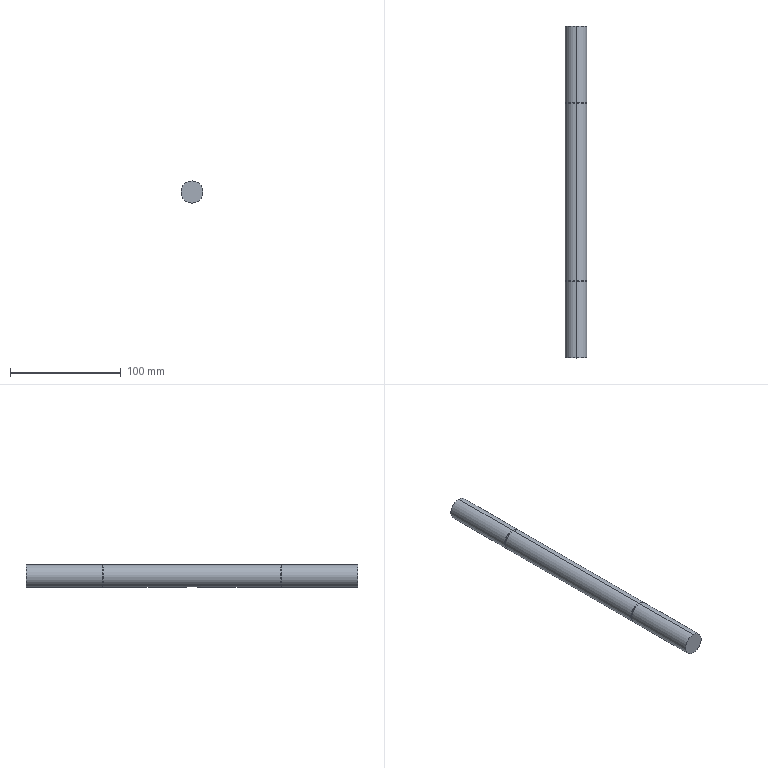Part | SolidWorks | features ICE 3, Chamfer 1, Extrusion 1 | 1 solid | 21 faces | box 20 x 300 x 20 mm | volume 93992 mm3 | cylinder 12 | plane 9 | commonest cylinder face diameters 20 x6 19 x4 6 x2
STEP:
#1=CARTESIAN_POINT('',(0.,300.,10.));
#2=VERTEX_POINT('',#1);
#3=CARTESIAN_POINT('',(0.,300.,-10.));
#4=VERTEX_POINT('',#3);
#5=CARTESIAN_POINT('',(0.,300.,0.));
#6=DIRECTION('',(0.,1.,0.));
#7=DIRECTION('',(0.,0.,1.));
#8=AXIS2_PLACEMENT_3D('',#5,#6,#7);
#9=CIRCLE('',#8,10.);
#10=EDGE_CURVE('',#2,#4,#9,.T.);
#11=ORIENTED_EDGE('',*,*,#10,.F.);
#12=CARTESIAN_POINT('',(0.,231.3,10.));
#13=VERTEX_POINT('',#12);
#14=CARTESIAN_POINT('',(0.,300.,10.));
#15=DIRECTION('',(0.,-1.,0.));
#16=VECTOR('',#15,1000.);
#17=LINE('',#14,#16);
#18=EDGE_CURVE('',#2,#13,#17,.T.);
#19=ORIENTED_EDGE('',*,*,#18,.T.);
#20=CARTESIAN_POINT('',(0.,231.3,-10.));
#21=VERTEX_POINT('',#20);
#22=CARTESIAN_POINT('',(0.,231.3,0.));
#23=DIRECTION('',(0.,1.,0.));
#24=DIRECTION('',(0.,0.,1.));
#25=AXIS2_PLACEMENT_3D('',#22,#23,#24);
#26=CIRCLE('',#25,10.);
#27=EDGE_CURVE('',#13,#21,#26,.T.);
#28=ORIENTED_EDGE('',*,*,#27,.T.);
#29=CARTESIAN_POINT('',(0.,300.,-10.));
#30=DIRECTION('',(0.,-1.,0.));
#31=VECTOR('',#30,1000.);
#32=LINE('',#29,#31);
#33=EDGE_CURVE('',#4,#21,#32,.T.);
#34=ORIENTED_EDGE('',*,*,#33,.F.);
#35=EDGE_LOOP('',(#11,#19,#28,#34));
#36=FACE_OUTER_BOUND('',#35,.T.);
#37=CARTESIAN_POINT('',(0.,300.,0.));
#38=DIRECTION('',(0.,-1.,0.));
#39=DIRECTION('',(0.,0.,-1.));
#40=AXIS2_PLACEMENT_3D('',#37,#38,#39);
#41=CYLINDRICAL_SURFACE('',#40,10.);
#42=ADVANCED_FACE('',(#36),#41,.T.);
#43=CARTESIAN_POINT('',(0.,231.3,9.5));
#44=VERTEX_POINT('',#43);
#45=CARTESIAN_POINT('',(0.,231.3,-9.5));
#46=VERTEX_POINT('',#45);
#47=CARTESIAN_POINT('',(0.,231.3,0.));
#48=DIRECTION('',(0.,1.,0.));
#49=DIRECTION('',(0.,0.,1.));
#50=AXIS2_PLACEMENT_3D('',#47,#48,#49);
#51=CIRCLE('',#50,9.5);
#52=EDGE_CURVE('',#44,#46,#51,.T.);
#53=ORIENTED_EDGE('',*,*,#52,.F.);
#54=CARTESIAN_POINT('',(0.,230.,9.5));
#55=VERTEX_POINT('',#54);
#56=CARTESIAN_POINT('',(0.,231.3,9.5));
#57=DIRECTION('',(0.,-1.,0.));
#58=VECTOR('',#57,1000.);
#59=LINE('',#56,#58);
#60=EDGE_CURVE('',#44,#55,#59,.T.);
#61=ORIENTED_EDGE('',*,*,#60,.T.);
#62=CARTESIAN_POINT('',(0.,230.,-9.5));
#63=VERTEX_POINT('',#62);
#64=CARTESIAN_POINT('',(0.,230.,0.));
#65=DIRECTION('',(0.,1.,0.));
#66=DIRECTION('',(0.,0.,1.));
#67=AXIS2_PLACEMENT_3D('',#64,#65,#66);
#68=CIRCLE('',#67,9.5);
#69=EDGE_CURVE('',#55,#63,#68,.T.);
#70=ORIENTED_EDGE('',*,*,#69,.T.);
#71=CARTESIAN_POINT('',(0.,231.3,-9.5));
#72=DIRECTION('',(0.,-1.,0.));
#73=VECTOR('',#72,1000.);
#74=LINE('',#71,#73);
#75=EDGE_CURVE('',#46,#63,#74,.T.);
#76=ORIENTED_EDGE('',*,*,#75,.F.);
#77=EDGE_LOOP('',(#53,#61,#70,#76));
#78=FACE_OUTER_BOUND('',#77,.T.);
#79=CARTESIAN_POINT('',(0.,231.3,0.));
#80=DIRECTION('',(0.,-1.,0.));
#81=DIRECTION('',(0.,0.,-1.));
#82=AXIS2_PLACEMENT_3D('',#79,#80,#81);
#83=CYLINDRICAL_SURFACE('',#82,9.5);
#84=ADVANCED_FACE('',(#78),#83,.T.);
#85=CARTESIAN_POINT('',(0.,68.7,-9.5));
#86=VERTEX_POINT('',#85);
#87=CARTESIAN_POINT('',(0.,68.7,9.5));
#88=VERTEX_POINT('',#87);
#89=CARTESIAN_POINT('',(0.,68.7,0.));
#90=DIRECTION('',(0.,-1.,0.));
#91=DIRECTION('',(0.,0.,-1.));
#92=AXIS2_PLACEMENT_3D('',#89,#90,#91);
#93=CIRCLE('',#92,9.5);
#94=EDGE_CURVE('',#86,#88,#93,.T.);
#95=ORIENTED_EDGE('',*,*,#94,.F.);
#96=CARTESIAN_POINT('',(0.,70.,-9.5));
#97=VERTEX_POINT('',#96);
#98=CARTESIAN_POINT('',(0.,68.7,-9.5));
#99=DIRECTION('',(0.,1.,0.));
#100=VECTOR('',#99,1000.);
#101=LINE('',#98,#100);
#102=EDGE_CURVE('',#86,#97,#101,.T.);
#103=ORIENTED_EDGE('',*,*,#102,.T.);
#104=CARTESIAN_POINT('',(0.,70.,9.5));
#105=VERTEX_POINT('',#104);
#106=CARTESIAN_POINT('',(0.,70.,0.));
#107=DIRECTION('',(0.,-1.,0.));
#108=DIRECTION('',(0.,0.,-1.));
#109=AXIS2_PLACEMENT_3D('',#106,#107,#108);
#110=CIRCLE('',#109,9.5);
#111=EDGE_CURVE('',#97,#105,#110,.T.);
#112=ORIENTED_EDGE('',*,*,#111,.T.);
#113=CARTESIAN_POINT('',(0.,68.7,9.5));
#114=DIRECTION('',(0.,1.,0.));
#115=VECTOR('',#114,1000.);
#116=LINE('',#113,#115);
#117=EDGE_CURVE('',#88,#105,#116,.T.);
#118=ORIENTED_EDGE('',*,*,#117,.F.);
#119=EDGE_LOOP('',(#95,#103,#112,#118));
#120=FACE_OUTER_BOUND('',#119,.T.);
#121=CARTESIAN_POINT('',(0.,68.7,0.));
#122=DIRECTION('',(0.,1.,0.));
#123=DIRECTION('',(0.,0.,1.));
#124=AXIS2_PLACEMENT_3D('',#121,#122,#123);
#125=CYLINDRICAL_SURFACE('',#124,9.5);
#126=ADVANCED_FACE('',(#120),#125,.T.);
#127=CARTESIAN_POINT('',(0.,68.7,-10.));
#128=VERTEX_POINT('',#127);
#129=CARTESIAN_POINT('',(0.,68.7,10.));
#130=VERTEX_POINT('',#129);
#131=CARTESIAN_POINT('',(0.,68.7,0.));
#132=DIRECTION('',(0.,-1.,0.));
#133=DIRECTION('',(0.,0.,-1.));
#134=AXIS2_PLACEMENT_3D('',#131,#132,#133);
#135=CIRCLE('',#134,10.);
#136=EDGE_CURVE('',#128,#130,#135,.T.);
#137=ORIENTED_EDGE('',*,*,#136,.T.);
#138=CARTESIAN_POINT('',(0.,0.,10.));
#139=VERTEX_POINT('',#138);
#140=CARTESIAN_POINT('',(0.,300.,10.));
#141=DIRECTION('',(0.,-1.,0.));
#142=VECTOR('',#141,1000.);
#143=LINE('',#140,#142);
#144=EDGE_CURVE('',#130,#139,#143,.T.);
#145=ORIENTED_EDGE('',*,*,#144,.T.);
#146=CARTESIAN_POINT('',(0.,0.,-10.));
#147=VERTEX_POINT('',#146);
#148=CARTESIAN_POINT('',(0.,0.,0.));
#149=DIRECTION('',(0.,1.,0.));
#150=DIRECTION('',(0.,0.,1.));
#151=AXIS2_PLACEMENT_3D('',#148,#149,#150);
#152=CIRCLE('',#151,10.);
#153=EDGE_CURVE('',#139,#147,#152,.T.);
#154=ORIENTED_EDGE('',*,*,#153,.T.);
#155=CARTESIAN_POINT('',(0.,300.,-10.));
#156=DIRECTION('',(0.,-1.,0.));
#157=VECTOR('',#156,1000.);
#158=LINE('',#155,#157);
#159=EDGE_CURVE('',#128,#147,#158,.T.);
#160=ORIENTED_EDGE('',*,*,#159,.F.);
#161=EDGE_LOOP('',(#137,#145,#154,#160));
#162=FACE_OUTER_BOUND('',#161,.T.);
#163=CARTESIAN_POINT('',(0.,300.,0.));
#164=DIRECTION('',(0.,-1.,0.));
#165=DIRECTION('',(0.,0.,-1.));
#166=AXIS2_PLACEMENT_3D('',#163,#164,#165);
#167=CYLINDRICAL_SURFACE('',#166,10.);
#168=ADVANCED_FACE('',(#162),#167,.T.);
#169=CARTESIAN_POINT('',(0.,230.,10.));
#170=VERTEX_POINT('',#169);
#171=CARTESIAN_POINT('',(0.,230.,-10.));
#172=VERTEX_POINT('',#171);
#173=CARTESIAN_POINT('',(0.,230.,0.));
#174=DIRECTION('',(0.,1.,0.));
#175=DIRECTION('',(0.,0.,1.));
#176=AXIS2_PLACEMENT_3D('',#173,#174,#175);
#177=CIRCLE('',#176,10.);
#178=EDGE_CURVE('',#170,#172,#177,.T.);
#179=ORIENTED_EDGE('',*,*,#178,.F.);
#180=CARTESIAN_POINT('',(0.,70.,10.));
#181=VERTEX_POINT('',#180);
#182=CARTESIAN_POINT('',(0.,300.,10.));
#183=DIRECTION('',(0.,-1.,0.));
#184=VECTOR('',#183,1000.);
#185=LINE('',#182,#184);
#186=EDGE_CURVE('',#170,#181,#185,.T.);
#187=ORIENTED_EDGE('',*,*,#186,.T.);
#188=CARTESIAN_POINT('',(0.,70.,-10.));
#189=VERTEX_POINT('',#188);
#190=CARTESIAN_POINT('',(0.,70.,0.));
#191=DIRECTION('',(0.,-1.,0.));
#192=DIRECTION('',(0.,0.,-1.));
#193=AXIS2_PLACEMENT_3D('',#190,#191,#192);
#194=CIRCLE('',#193,10.);
#195=EDGE_CURVE('',#189,#181,#194,.T.);
#196=ORIENTED_EDGE('',*,*,#195,.F.);
#197=CARTESIAN_POINT('',(0.,145.,-10.));
#198=VERTEX_POINT('',#197);
#199=CARTESIAN_POINT('',(0.,300.,-10.));
#200=DIRECTION('',(0.,-1.,0.));
#201=VECTOR('',#200,1000.);
#202=LINE('',#199,#201);
#203=EDGE_CURVE('',#198,#189,#202,.T.);
#204=ORIENTED_EDGE('',*,*,#203,.F.);
#205=CARTESIAN_POINT('',(3.,148.,-9.539));
#206=VERTEX_POINT('',#205);
#207=CARTESIAN_POINT('',(0.,145.,-10.));
#208=CARTESIAN_POINT('',(0.1968,145.,-10.));
#209=CARTESIAN_POINT('',(0.3967,145.02,-9.994));
#210=CARTESIAN_POINT('',(0.7821,145.097,-9.971));
#211=CARTESIAN_POINT('',(0.9695,145.154,-9.955));
#212=CARTESIAN_POINT('',(1.334,145.306,-9.912));
#213=CARTESIAN_POINT('',(1.507,145.399,-9.887));
#214=CARTESIAN_POINT('',(1.831,145.616,-9.832));
#215=CARTESIAN_POINT('',(1.983,145.741,-9.802));
#216=CARTESIAN_POINT('',(2.26,146.017,-9.742));
#217=CARTESIAN_POINT('',(2.383,146.167,-9.713));
#218=CARTESIAN_POINT('',(2.6,146.491,-9.657));
#219=CARTESIAN_POINT('',(2.694,146.667,-9.63));
#220=CARTESIAN_POINT('',(2.845,147.028,-9.587));
#221=CARTESIAN_POINT('',(2.902,147.215,-9.57));
#222=CARTESIAN_POINT('',(2.98,147.601,-9.546));
#223=CARTESIAN_POINT('',(3.,147.801,-9.539));
#224=CARTESIAN_POINT('',(3.,148.,-9.539));
#225=B_SPLINE_CURVE_WITH_KNOTS('',3,(#207,#208,#209,#210,#211,#212,#213,#214,#215,#216,#217,#218,#219,#220,#221,#222,#223,#224),.UNSPECIFIED.,.F.,.F.,(4,2,2,2,2,2,2,2,4),(0.004718,0.005307,0.005896,0.006485,0.007074,0.007663,0.008252,0.008842,0.009431),.UNSPECIFIED.);
#226=EDGE_CURVE('',#198,#206,#225,.T.);
#227=ORIENTED_EDGE('',*,*,#226,.T.);
#228=CARTESIAN_POINT('',(3.,152.,-9.539));
#229=VERTEX_POINT('',#228);
#230=CARTESIAN_POINT('',(3.,300.,-9.539));
#231=DIRECTION('',(0.,1.,0.));
#232=VECTOR('',#231,1000.);
#233=LINE('',#230,#232);
#234=EDGE_CURVE('',#206,#229,#233,.T.);
#235=ORIENTED_EDGE('',*,*,#234,.T.);
#236=CARTESIAN_POINT('',(0.,155.,-10.));
#237=VERTEX_POINT('',#236);
#238=CARTESIAN_POINT('',(3.,152.,-9.539));
#239=CARTESIAN_POINT('',(3.,152.2,-9.539));
#240=CARTESIAN_POINT('',(2.98,152.395,-9.546));
#241=CARTESIAN_POINT('',(2.903,152.781,-9.569));
#242=CARTESIAN_POINT('',(2.845,152.972,-9.587));
#243=CARTESIAN_POINT('',(2.694,153.335,-9.631));
#244=CARTESIAN_POINT('',(2.602,153.506,-9.656));
#245=CARTESIAN_POINT('',(2.384,153.832,-9.712));
#246=CARTESIAN_POINT('',(2.258,153.985,-9.743));
#247=CARTESIAN_POINT('',(1.845,154.397,-9.832));
#248=CARTESIAN_POINT('',(1.512,154.62,-9.892));
#249=CARTESIAN_POINT('',(0.971,154.845,-9.954));
#250=CARTESIAN_POINT('',(0.7806,154.903,-9.971));
#251=CARTESIAN_POINT('',(0.3926,154.981,-9.994));
#252=CARTESIAN_POINT('',(0.197,155.,-10.));
#253=CARTESIAN_POINT('',(0.,155.,-10.));
#254=B_SPLINE_CURVE_WITH_KNOTS('',3,(#238,#239,#240,#241,#242,#243,#244,#245,#246,#247,#248,#249,#250,#251,#252,#253),.UNSPECIFIED.,.F.,.F.,(4,2,2,2,2,2,2,4),(0.,0.0005898,0.00118,0.001769,0.002359,0.003539,0.004128,0.004718),.UNSPECIFIED.);
#255=EDGE_CURVE('',#229,#237,#254,.T.);
#256=ORIENTED_EDGE('',*,*,#255,.T.);
#257=CARTESIAN_POINT('',(0.,300.,-10.));
#258=DIRECTION('',(0.,-1.,0.));
#259=VECTOR('',#258,1000.);
#260=LINE('',#257,#259);
#261=EDGE_CURVE('',#172,#237,#260,.T.);
#262=ORIENTED_EDGE('',*,*,#261,.F.);
#263=EDGE_LOOP('',(#179,#187,#196,#204,#227,#235,#256,#262));
#264=FACE_OUTER_BOUND('',#263,.T.);
#265=CARTESIAN_POINT('',(0.,300.,0.));
#266=DIRECTION('',(0.,-1.,0.));
#267=DIRECTION('',(0.,0.,-1.));
#268=AXIS2_PLACEMENT_3D('',#265,#266,#267);
#269=CYLINDRICAL_SURFACE('',#268,10.);
#270=ADVANCED_FACE('',(#264),#269,.T.);
#271=ORIENTED_EDGE('',*,*,#186,.F.);
#272=CARTESIAN_POINT('',(0.,230.,0.));
#273=DIRECTION('',(0.,1.,0.));
#274=DIRECTION('',(0.,0.,1.));
#275=AXIS2_PLACEMENT_3D('',#272,#273,#274);
#276=CIRCLE('',#275,10.);
#277=EDGE_CURVE('',#172,#170,#276,.T.);
#278=ORIENTED_EDGE('',*,*,#277,.F.);
#279=ORIENTED_EDGE('',*,*,#261,.T.);
#280=CARTESIAN_POINT('',(-3.,152.,-9.539));
#281=VERTEX_POINT('',#280);
#282=CARTESIAN_POINT('',(0.,155.,-10.));
#283=CARTESIAN_POINT('',(-0.1968,155.,-10.));
#284=CARTESIAN_POINT('',(-0.3967,154.98,-9.994));
#285=CARTESIAN_POINT('',(-0.7821,154.903,-9.971));
#286=CARTESIAN_POINT('',(-0.9695,154.846,-9.955));
#287=CARTESIAN_POINT('',(-1.334,154.694,-9.912));
#288=CARTESIAN_POINT('',(-1.507,154.601,-9.887));
#289=CARTESIAN_POINT('',(-1.831,154.384,-9.832));
#290=CARTESIAN_POINT('',(-1.983,154.259,-9.802));
#291=CARTESIAN_POINT('',(-2.26,153.983,-9.742));
#292=CARTESIAN_POINT('',(-2.383,153.833,-9.713));
#293=CARTESIAN_POINT('',(-2.6,153.509,-9.657));
#294=CARTESIAN_POINT('',(-2.694,153.333,-9.63));
#295=CARTESIAN_POINT('',(-2.845,152.972,-9.587));
#296=CARTESIAN_POINT('',(-2.902,152.785,-9.57));
#297=CARTESIAN_POINT('',(-2.98,152.399,-9.546));
#298=CARTESIAN_POINT('',(-3.,152.199,-9.539));
#299=CARTESIAN_POINT('',(-3.,152.,-9.539));
#300=B_SPLINE_CURVE_WITH_KNOTS('',3,(#282,#283,#284,#285,#286,#287,#288,#289,#290,#291,#292,#293,#294,#295,#296,#297,#298,#299),.UNSPECIFIED.,.F.,.F.,(4,2,2,2,2,2,2,2,4),(0.004718,0.005307,0.005896,0.006485,0.007074,0.007663,0.008252,0.008842,0.009431),.UNSPECIFIED.);
#301=EDGE_CURVE('',#237,#281,#300,.T.);
#302=ORIENTED_EDGE('',*,*,#301,.T.);
#303=CARTESIAN_POINT('',(-3.,148.,-9.539));
#304=VERTEX_POINT('',#303);
#305=CARTESIAN_POINT('',(-3.,300.,-9.539));
#306=DIRECTION('',(0.,-1.,0.));
#307=VECTOR('',#306,1000.);
#308=LINE('',#305,#307);
#309=EDGE_CURVE('',#281,#304,#308,.T.);
#310=ORIENTED_EDGE('',*,*,#309,.T.);
#311=CARTESIAN_POINT('',(-3.,148.,-9.539));
#312=CARTESIAN_POINT('',(-3.,147.8,-9.539));
#313=CARTESIAN_POINT('',(-2.98,147.605,-9.546));
#314=CARTESIAN_POINT('',(-2.903,147.219,-9.569));
#315=CARTESIAN_POINT('',(-2.845,147.028,-9.587));
#316=CARTESIAN_POINT('',(-2.694,146.665,-9.631));
#317=CARTESIAN_POINT('',(-2.602,146.494,-9.656));
#318=CARTESIAN_POINT('',(-2.384,146.168,-9.712));
#319=CARTESIAN_POINT('',(-2.258,146.015,-9.743));
#320=CARTESIAN_POINT('',(-1.845,145.603,-9.832));
#321=CARTESIAN_POINT('',(-1.512,145.38,-9.892));
#322=CARTESIAN_POINT('',(-0.971,145.155,-9.954));
#323=CARTESIAN_POINT('',(-0.7806,145.097,-9.971));
#324=CARTESIAN_POINT('',(-0.3926,145.019,-9.994));
#325=CARTESIAN_POINT('',(-0.197,145.,-10.));
#326=CARTESIAN_POINT('',(0.,145.,-10.));
#327=B_SPLINE_CURVE_WITH_KNOTS('',3,(#311,#312,#313,#314,#315,#316,#317,#318,#319,#320,#321,#322,#323,#324,#325,#326),.UNSPECIFIED.,.F.,.F.,(4,2,2,2,2,2,2,4),(0.,0.0005898,0.00118,0.001769,0.002359,0.003539,0.004128,0.004718),.UNSPECIFIED.);
#328=EDGE_CURVE('',#304,#198,#327,.T.);
#329=ORIENTED_EDGE('',*,*,#328,.T.);
#330=ORIENTED_EDGE('',*,*,#203,.T.);
#331=CARTESIAN_POINT('',(0.,70.,0.));
#332=DIRECTION('',(0.,-1.,0.));
#333=DIRECTION('',(0.,0.,-1.));
#334=AXIS2_PLACEMENT_3D('',#331,#332,#333);
#335=CIRCLE('',#334,10.);
#336=EDGE_CURVE('',#181,#189,#335,.T.);
#337=ORIENTED_EDGE('',*,*,#336,.F.);
#338=EDGE_LOOP('',(#271,#278,#279,#302,#310,#329,#330,#337));
#339=FACE_OUTER_BOUND('',#338,.T.);
#340=CARTESIAN_POINT('',(0.,300.,0.));
#341=DIRECTION('',(0.,-1.,0.));
#342=DIRECTION('',(0.,0.,-1.));
#343=AXIS2_PLACEMENT_3D('',#340,#341,#342);
#344=CYLINDRICAL_SURFACE('',#343,10.);
#345=ADVANCED_FACE('',(#339),#344,.T.);
#346=ORIENTED_EDGE('',*,*,#144,.F.);
#347=CARTESIAN_POINT('',(0.,68.7,0.));
#348=DIRECTION('',(0.,-1.,0.));
#349=DIRECTION('',(0.,0.,-1.));
#350=AXIS2_PLACEMENT_3D('',#347,#348,#349);
#351=CIRCLE('',#350,10.);
#352=EDGE_CURVE('',#130,#128,#351,.T.);
#353=ORIENTED_EDGE('',*,*,#352,.T.);
#354=ORIENTED_EDGE('',*,*,#159,.T.);
#355=CARTESIAN_POINT('',(0.,0.,0.));
#356=DIRECTION('',(0.,1.,0.));
#357=DIRECTION('',(0.,0.,1.));
#358=AXIS2_PLACEMENT_3D('',#355,#356,#357);
#359=CIRCLE('',#358,10.);
#360=EDGE_CURVE('',#147,#139,#359,.T.);
#361=ORIENTED_EDGE('',*,*,#360,.T.);
#362=EDGE_LOOP('',(#346,#353,#354,#361));
#363=FACE_OUTER_BOUND('',#362,.T.);
#364=CARTESIAN_POINT('',(0.,300.,0.));
#365=DIRECTION('',(0.,-1.,0.));
#366=DIRECTION('',(0.,0.,-1.));
#367=AXIS2_PLACEMENT_3D('',#364,#365,#366);
#368=CYLINDRICAL_SURFACE('',#367,10.);
#369=ADVANCED_FACE('',(#363),#368,.T.);
#370=ORIENTED_EDGE('',*,*,#360,.F.);
#371=ORIENTED_EDGE('',*,*,#153,.F.);
#372=EDGE_LOOP('',(#370,#371));
#373=FACE_OUTER_BOUND('',#372,.T.);
#374=CARTESIAN_POINT('',(0.,0.,0.));
#375=DIRECTION('',(0.,1.,0.));
#376=DIRECTION('',(0.,0.,1.));
#377=AXIS2_PLACEMENT_3D('',#374,#375,#376);
#378=PLANE('',#377);
#379=ADVANCED_FACE('',(#373),#378,.F.);
#380=ORIENTED_EDGE('',*,*,#136,.F.);
#381=ORIENTED_EDGE('',*,*,#352,.F.);
#382=EDGE_LOOP('',(#380,#381));
#383=FACE_OUTER_BOUND('',#382,.T.);
#384=CARTESIAN_POINT('',(0.,68.7,0.));
#385=DIRECTION('',(0.,-1.,0.));
#386=DIRECTION('',(0.,0.,-1.));
#387=AXIS2_PLACEMENT_3D('',#384,#385,#386);
#388=CIRCLE('',#387,9.5);
#389=EDGE_CURVE('',#88,#86,#388,.T.);
#390=ORIENTED_EDGE('',*,*,#389,.T.);
#391=ORIENTED_EDGE('',*,*,#94,.T.);
#392=EDGE_LOOP('',(#390,#391));
#393=FACE_BOUND('',#392,.T.);
#394=CARTESIAN_POINT('',(0.,68.7,0.));
#395=DIRECTION('',(0.,-1.,0.));
#396=DIRECTION('',(0.,0.,-1.));
#397=AXIS2_PLACEMENT_3D('',#394,#395,#396);
#398=PLANE('',#397);
#399=ADVANCED_FACE('',(#383,#393),#398,.F.);
#400=ORIENTED_EDGE('',*,*,#195,.T.);
#401=ORIENTED_EDGE('',*,*,#336,.T.);
#402=EDGE_LOOP('',(#400,#401));
#403=FACE_OUTER_BOUND('',#402,.T.);
#404=CARTESIAN_POINT('',(0.,70.,0.));
#405=DIRECTION('',(0.,-1.,0.));
#406=DIRECTION('',(0.,0.,-1.));
#407=AXIS2_PLACEMENT_3D('',#404,#405,#406);
#408=CIRCLE('',#407,9.5);
#409=EDGE_CURVE('',#105,#97,#408,.T.);
#410=ORIENTED_EDGE('',*,*,#409,.F.);
#411=ORIENTED_EDGE('',*,*,#111,.F.);
#412=EDGE_LOOP('',(#410,#411));
#413=FACE_BOUND('',#412,.T.);
#414=CARTESIAN_POINT('',(0.,70.,0.));
#415=DIRECTION('',(0.,-1.,0.));
#416=DIRECTION('',(0.,0.,-1.));
#417=AXIS2_PLACEMENT_3D('',#414,#415,#416);
#418=PLANE('',#417);
#419=ADVANCED_FACE('',(#403,#413),#418,.T.);
#420=ORIENTED_EDGE('',*,*,#102,.F.);
#421=ORIENTED_EDGE('',*,*,#389,.F.);
#422=ORIENTED_EDGE('',*,*,#117,.T.);
#423=ORIENTED_EDGE('',*,*,#409,.T.);
#424=EDGE_LOOP('',(#420,#421,#422,#423));
#425=FACE_OUTER_BOUND('',#424,.T.);
#426=CARTESIAN_POINT('',(0.,68.7,0.));
#427=DIRECTION('',(0.,1.,0.));
#428=DIRECTION('',(0.,0.,1.));
#429=AXIS2_PLACEMENT_3D('',#426,#427,#428);
#430=CYLINDRICAL_SURFACE('',#429,9.5);
#431=ADVANCED_FACE('',(#425),#430,.T.);
#432=CARTESIAN_POINT('',(0.,231.3,0.));
#433=DIRECTION('',(0.,1.,0.));
#434=DIRECTION('',(0.,0.,1.));
#435=AXIS2_PLACEMENT_3D('',#432,#433,#434);
#436=CIRCLE('',#435,10.);
#437=EDGE_CURVE('',#21,#13,#436,.T.);
#438=ORIENTED_EDGE('',*,*,#437,.F.);
#439=ORIENTED_EDGE('',*,*,#27,.F.);
#440=EDGE_LOOP('',(#438,#439));
#441=FACE_OUTER_BOUND('',#440,.T.);
#442=CARTESIAN_POINT('',(0.,231.3,0.));
#443=DIRECTION('',(0.,1.,0.));
#444=DIRECTION('',(0.,0.,1.));
#445=AXIS2_PLACEMENT_3D('',#442,#443,#444);
#446=CIRCLE('',#445,9.5);
#447=EDGE_CURVE('',#46,#44,#446,.T.);
#448=ORIENTED_EDGE('',*,*,#447,.T.);
#449=ORIENTED_EDGE('',*,*,#52,.T.);
#450=EDGE_LOOP('',(#448,#449));
#451=FACE_BOUND('',#450,.T.);
#452=CARTESIAN_POINT('',(0.,231.3,0.));
#453=DIRECTION('',(0.,1.,0.));
#454=DIRECTION('',(0.,0.,1.));
#455=AXIS2_PLACEMENT_3D('',#452,#453,#454);
#456=PLANE('',#455);
#457=ADVANCED_FACE('',(#441,#451),#456,.F.);
#458=ORIENTED_EDGE('',*,*,#277,.T.);
#459=ORIENTED_EDGE('',*,*,#178,.T.);
#460=EDGE_LOOP('',(#458,#459));
#461=FACE_OUTER_BOUND('',#460,.T.);
#462=CARTESIAN_POINT('',(0.,230.,0.));
#463=DIRECTION('',(0.,1.,0.));
#464=DIRECTION('',(0.,0.,1.));
#465=AXIS2_PLACEMENT_3D('',#462,#463,#464);
#466=CIRCLE('',#465,9.5);
#467=EDGE_CURVE('',#63,#55,#466,.T.);
#468=ORIENTED_EDGE('',*,*,#467,.F.);
#469=ORIENTED_EDGE('',*,*,#69,.F.);
#470=EDGE_LOOP('',(#468,#469));
#471=FACE_BOUND('',#470,.T.);
#472=CARTESIAN_POINT('',(0.,230.,0.));
#473=DIRECTION('',(0.,1.,0.));
#474=DIRECTION('',(0.,0.,1.));
#475=AXIS2_PLACEMENT_3D('',#472,#473,#474);
#476=PLANE('',#475);
#477=ADVANCED_FACE('',(#461,#471),#476,.T.);
#478=ORIENTED_EDGE('',*,*,#60,.F.);
#479=ORIENTED_EDGE('',*,*,#447,.F.);
#480=ORIENTED_EDGE('',*,*,#75,.T.);
#481=ORIENTED_EDGE('',*,*,#467,.T.);
#482=EDGE_LOOP('',(#478,#479,#480,#481));
#483=FACE_OUTER_BOUND('',#482,.T.);
#484=CARTESIAN_POINT('',(0.,231.3,0.));
#485=DIRECTION('',(0.,-1.,0.));
#486=DIRECTION('',(0.,0.,-1.));
#487=AXIS2_PLACEMENT_3D('',#484,#485,#486);
#488=CYLINDRICAL_SURFACE('',#487,9.5);
#489=ADVANCED_FACE('',(#483),#488,.T.);
#490=CARTESIAN_POINT('',(0.,300.,0.));
#491=DIRECTION('',(0.,1.,0.));
#492=DIRECTION('',(0.,0.,1.));
#493=AXIS2_PLACEMENT_3D('',#490,#491,#492);
#494=CIRCLE('',#493,10.);
#495=EDGE_CURVE('',#4,#2,#494,.T.);
#496=ORIENTED_EDGE('',*,*,#495,.T.);
#497=ORIENTED_EDGE('',*,*,#10,.T.);
#498=EDGE_LOOP('',(#496,#497));
#499=FACE_OUTER_BOUND('',#498,.T.);
#500=CARTESIAN_POINT('',(0.,300.,0.));
#501=DIRECTION('',(0.,1.,0.));
#502=DIRECTION('',(0.,0.,1.));
#503=AXIS2_PLACEMENT_3D('',#500,#501,#502);
#504=PLANE('',#503);
#505=ADVANCED_FACE('',(#499),#504,.T.);
#506=ORIENTED_EDGE('',*,*,#18,.F.);
#507=ORIENTED_EDGE('',*,*,#495,.F.);
#508=ORIENTED_EDGE('',*,*,#33,.T.);
#509=ORIENTED_EDGE('',*,*,#437,.T.);
#510=EDGE_LOOP('',(#506,#507,#508,#509));
#511=FACE_OUTER_BOUND('',#510,.T.);
#512=CARTESIAN_POINT('',(0.,300.,0.));
#513=DIRECTION('',(0.,-1.,0.));
#514=DIRECTION('',(0.,0.,-1.));
#515=AXIS2_PLACEMENT_3D('',#512,#513,#514);
#516=CYLINDRICAL_SURFACE('',#515,10.);
#517=ADVANCED_FACE('',(#511),#516,.T.);
#518=CARTESIAN_POINT('',(-3.,148.,-6.5));
#519=VERTEX_POINT('',#518);
#520=CARTESIAN_POINT('',(-3.,148.,-6.5));
#521=DIRECTION('',(0.,0.,-1.));
#522=VECTOR('',#521,1000.);
#523=LINE('',#520,#522);
#524=EDGE_CURVE('',#519,#304,#523,.T.);
#525=ORIENTED_EDGE('',*,*,#524,.F.);
#526=CARTESIAN_POINT('',(3.,148.,-6.5));
#527=VERTEX_POINT('',#526);
#528=CARTESIAN_POINT('',(0.,148.,-6.5));
#529=DIRECTION('',(0.,0.,-1.));
#530=DIRECTION('',(-1.,0.,0.));
#531=AXIS2_PLACEMENT_3D('',#528,#529,#530);
#532=CIRCLE('',#531,3.);
#533=EDGE_CURVE('',#527,#519,#532,.T.);
#534=ORIENTED_EDGE('',*,*,#533,.F.);
#535=CARTESIAN_POINT('',(3.,148.,-6.5));
#536=DIRECTION('',(0.,0.,-1.));
#537=VECTOR('',#536,1000.);
#538=LINE('',#535,#537);
#539=EDGE_CURVE('',#527,#206,#538,.T.);
#540=ORIENTED_EDGE('',*,*,#539,.T.);
#541=ORIENTED_EDGE('',*,*,#226,.F.);
#542=ORIENTED_EDGE('',*,*,#328,.F.);
#543=EDGE_LOOP('',(#525,#534,#540,#541,#542));
#544=FACE_OUTER_BOUND('',#543,.T.);
#545=CARTESIAN_POINT('',(0.,148.,-6.5));
#546=DIRECTION('',(0.,0.,-1.));
#547=DIRECTION('',(-1.,0.,0.));
#548=AXIS2_PLACEMENT_3D('',#545,#546,#547);
#549=CYLINDRICAL_SURFACE('',#548,3.);
#550=ADVANCED_FACE('',(#544),#549,.F.);
#551=ORIENTED_EDGE('',*,*,#539,.F.);
#552=CARTESIAN_POINT('',(3.,152.,-6.5));
#553=VERTEX_POINT('',#552);
#554=CARTESIAN_POINT('',(3.,148.,-6.5));
#555=DIRECTION('',(0.,-1.,0.));
#556=VECTOR('',#555,1000.);
#557=LINE('',#554,#556);
#558=EDGE_CURVE('',#553,#527,#557,.T.);
#559=ORIENTED_EDGE('',*,*,#558,.F.);
#560=CARTESIAN_POINT('',(3.,152.,-6.5));
#561=DIRECTION('',(0.,0.,-1.));
#562=VECTOR('',#561,1000.);
#563=LINE('',#560,#562);
#564=EDGE_CURVE('',#553,#229,#563,.T.);
#565=ORIENTED_EDGE('',*,*,#564,.T.);
#566=ORIENTED_EDGE('',*,*,#234,.F.);
#567=EDGE_LOOP('',(#551,#559,#565,#566));
#568=FACE_OUTER_BOUND('',#567,.T.);
#569=CARTESIAN_POINT('',(3.,148.,-6.5));
#570=DIRECTION('',(1.,0.,0.));
#571=DIRECTION('',(0.,0.,-1.));
#572=AXIS2_PLACEMENT_3D('',#569,#570,#571);
#573=PLANE('',#572);
#574=ADVANCED_FACE('',(#568),#573,.F.);
#575=ORIENTED_EDGE('',*,*,#564,.F.);
#576=CARTESIAN_POINT('',(-3.,152.,-6.5));
#577=VERTEX_POINT('',#576);
#578=CARTESIAN_POINT('',(0.,152.,-6.5));
#579=DIRECTION('',(0.,0.,-1.));
#580=DIRECTION('',(-1.,0.,0.));
#581=AXIS2_PLACEMENT_3D('',#578,#579,#580);
#582=CIRCLE('',#581,3.);
#583=EDGE_CURVE('',#577,#553,#582,.T.);
#584=ORIENTED_EDGE('',*,*,#583,.F.);
#585=CARTESIAN_POINT('',(-3.,152.,-6.5));
#586=DIRECTION('',(0.,0.,-1.));
#587=VECTOR('',#586,1000.);
#588=LINE('',#585,#587);
#589=EDGE_CURVE('',#577,#281,#588,.T.);
#590=ORIENTED_EDGE('',*,*,#589,.T.);
#591=ORIENTED_EDGE('',*,*,#301,.F.);
#592=ORIENTED_EDGE('',*,*,#255,.F.);
#593=EDGE_LOOP('',(#575,#584,#590,#591,#592));
#594=FACE_OUTER_BOUND('',#593,.T.);
#595=CARTESIAN_POINT('',(0.,152.,-6.5));
#596=DIRECTION('',(0.,0.,-1.));
#597=DIRECTION('',(-1.,0.,0.));
#598=AXIS2_PLACEMENT_3D('',#595,#596,#597);
#599=CYLINDRICAL_SURFACE('',#598,3.);
#600=ADVANCED_FACE('',(#594),#599,.F.);
#601=ORIENTED_EDGE('',*,*,#589,.F.);
#602=CARTESIAN_POINT('',(-3.,148.,-6.5));
#603=DIRECTION('',(0.,1.,0.));
#604=VECTOR('',#603,1000.);
#605=LINE('',#602,#604);
#606=EDGE_CURVE('',#519,#577,#605,.T.);
#607=ORIENTED_EDGE('',*,*,#606,.F.);
#608=ORIENTED_EDGE('',*,*,#524,.T.);
#609=ORIENTED_EDGE('',*,*,#309,.F.);
#610=EDGE_LOOP('',(#601,#607,#608,#609));
#611=FACE_OUTER_BOUND('',#610,.T.);
#612=CARTESIAN_POINT('',(-3.,148.,-6.5));
#613=DIRECTION('',(-1.,0.,0.));
#614=DIRECTION('',(0.,0.,1.));
#615=AXIS2_PLACEMENT_3D('',#612,#613,#614);
#616=PLANE('',#615);
#617=ADVANCED_FACE('',(#611),#616,.F.);
#618=ORIENTED_EDGE('',*,*,#533,.T.);
#619=ORIENTED_EDGE('',*,*,#606,.T.);
#620=ORIENTED_EDGE('',*,*,#583,.T.);
#621=ORIENTED_EDGE('',*,*,#558,.T.);
#622=EDGE_LOOP('',(#618,#619,#620,#621));
#623=FACE_OUTER_BOUND('',#622,.T.);
#624=CARTESIAN_POINT('',(0.,148.,-6.5));
#625=DIRECTION('',(0.,0.,-1.));
#626=DIRECTION('',(-1.,0.,0.));
#627=AXIS2_PLACEMENT_3D('',#624,#625,#626);
#628=PLANE('',#627);
#629=ADVANCED_FACE('',(#623),#628,.T.);
#630=CLOSED_SHELL('',(#42,#84,#126,#168,#270,#345,#369,#379,#399,#419,#431,#457,#477,#489,#505,#517,#550,#574,#600,#617,#629));
#631=MANIFOLD_SOLID_BREP('',#630);
#632=CARTESIAN_POINT('',(0.,0.,0.));
#633=DIRECTION('',(0.,0.,1.));
#634=DIRECTION('',(1.,0.,0.));
#635=AXIS2_PLACEMENT_3D('',#632,#633,#634);
#636=(LENGTH_UNIT()NAMED_UNIT(*)SI_UNIT(.MILLI.,.METRE.));
#637=UNCERTAINTY_MEASURE_WITH_UNIT(LENGTH_MEASURE(0.00001),#636,'','');
#638=(NAMED_UNIT(*)PLANE_ANGLE_UNIT()SI_UNIT($,.RADIAN.));
#639=(NAMED_UNIT(*)SI_UNIT($,.STERADIAN.)SOLID_ANGLE_UNIT());
#640=(GEOMETRIC_REPRESENTATION_CONTEXT(3)GLOBAL_UNCERTAINTY_ASSIGNED_CONTEXT((#637))GLOBAL_UNIT_ASSIGNED_CONTEXT((#636,#638,#639))REPRESENTATION_CONTEXT('',''));
#641=ADVANCED_BREP_SHAPE_REPRESENTATION('',(#631,#635),#640);